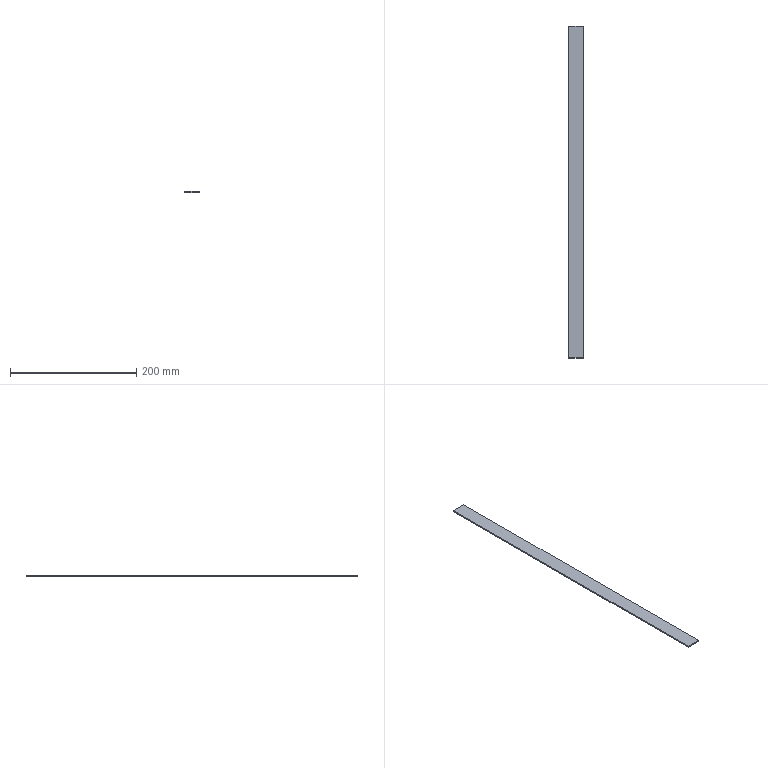Part | SolidWorks | features FlatPattern 1, SMBaseFlange 1, SheetMetal 1 | 1 solid | 6 faces | box 23 x 526 x 2 mm | volume 24196 mm3 | plane 6
STEP:
#1=CARTESIAN_POINT('',(11.5,-263.,0.));
#2=VERTEX_POINT('',#1);
#3=CARTESIAN_POINT('',(11.5,263.,0.));
#4=VERTEX_POINT('',#3);
#5=CARTESIAN_POINT('',(11.5,-263.,0.));
#6=DIRECTION('',(0.,1.,0.));
#7=VECTOR('',#6,1000.);
#8=LINE('',#5,#7);
#9=EDGE_CURVE('',#2,#4,#8,.T.);
#10=ORIENTED_EDGE('',*,*,#9,.F.);
#11=CARTESIAN_POINT('',(11.5,-263.,-2.));
#12=VERTEX_POINT('',#11);
#13=CARTESIAN_POINT('',(11.5,-263.,-2.));
#14=DIRECTION('',(0.,0.,1.));
#15=VECTOR('',#14,1000.);
#16=LINE('',#13,#15);
#17=EDGE_CURVE('',#12,#2,#16,.T.);
#18=ORIENTED_EDGE('',*,*,#17,.F.);
#19=CARTESIAN_POINT('',(11.5,263.,-2.));
#20=VERTEX_POINT('',#19);
#21=CARTESIAN_POINT('',(11.5,-263.,-2.));
#22=DIRECTION('',(0.,1.,0.));
#23=VECTOR('',#22,1000.);
#24=LINE('',#21,#23);
#25=EDGE_CURVE('',#12,#20,#24,.T.);
#26=ORIENTED_EDGE('',*,*,#25,.T.);
#27=CARTESIAN_POINT('',(11.5,263.,-2.));
#28=DIRECTION('',(0.,0.,1.));
#29=VECTOR('',#28,1000.);
#30=LINE('',#27,#29);
#31=EDGE_CURVE('',#20,#4,#30,.T.);
#32=ORIENTED_EDGE('',*,*,#31,.T.);
#33=EDGE_LOOP('',(#10,#18,#26,#32));
#34=FACE_OUTER_BOUND('',#33,.T.);
#35=CARTESIAN_POINT('',(11.5,-263.,-2.));
#36=DIRECTION('',(1.,0.,0.));
#37=DIRECTION('',(0.,0.,-1.));
#38=AXIS2_PLACEMENT_3D('',#35,#36,#37);
#39=PLANE('',#38);
#40=ADVANCED_FACE('',(#34),#39,.T.);
#41=CARTESIAN_POINT('',(-11.5,-263.,0.));
#42=VERTEX_POINT('',#41);
#43=CARTESIAN_POINT('',(-11.5,-263.,0.));
#44=DIRECTION('',(1.,0.,0.));
#45=VECTOR('',#44,1000.);
#46=LINE('',#43,#45);
#47=EDGE_CURVE('',#42,#2,#46,.T.);
#48=ORIENTED_EDGE('',*,*,#47,.F.);
#49=CARTESIAN_POINT('',(-11.5,-263.,-2.));
#50=VERTEX_POINT('',#49);
#51=CARTESIAN_POINT('',(-11.5,-263.,-2.));
#52=DIRECTION('',(0.,0.,1.));
#53=VECTOR('',#52,1000.);
#54=LINE('',#51,#53);
#55=EDGE_CURVE('',#50,#42,#54,.T.);
#56=ORIENTED_EDGE('',*,*,#55,.F.);
#57=CARTESIAN_POINT('',(-11.5,-263.,-2.));
#58=DIRECTION('',(1.,0.,0.));
#59=VECTOR('',#58,1000.);
#60=LINE('',#57,#59);
#61=EDGE_CURVE('',#50,#12,#60,.T.);
#62=ORIENTED_EDGE('',*,*,#61,.T.);
#63=ORIENTED_EDGE('',*,*,#17,.T.);
#64=EDGE_LOOP('',(#48,#56,#62,#63));
#65=FACE_OUTER_BOUND('',#64,.T.);
#66=CARTESIAN_POINT('',(-11.5,-263.,-2.));
#67=DIRECTION('',(0.,-1.,0.));
#68=DIRECTION('',(0.,0.,-1.));
#69=AXIS2_PLACEMENT_3D('',#66,#67,#68);
#70=PLANE('',#69);
#71=ADVANCED_FACE('',(#65),#70,.T.);
#72=CARTESIAN_POINT('',(-11.5,263.,0.));
#73=VERTEX_POINT('',#72);
#74=CARTESIAN_POINT('',(-11.5,-263.,0.));
#75=DIRECTION('',(0.,-1.,0.));
#76=VECTOR('',#75,1000.);
#77=LINE('',#74,#76);
#78=EDGE_CURVE('',#73,#42,#77,.T.);
#79=ORIENTED_EDGE('',*,*,#78,.F.);
#80=CARTESIAN_POINT('',(-11.5,263.,-2.));
#81=VERTEX_POINT('',#80);
#82=CARTESIAN_POINT('',(-11.5,263.,-2.));
#83=DIRECTION('',(0.,0.,1.));
#84=VECTOR('',#83,1000.);
#85=LINE('',#82,#84);
#86=EDGE_CURVE('',#81,#73,#85,.T.);
#87=ORIENTED_EDGE('',*,*,#86,.F.);
#88=CARTESIAN_POINT('',(-11.5,-263.,-2.));
#89=DIRECTION('',(0.,-1.,0.));
#90=VECTOR('',#89,1000.);
#91=LINE('',#88,#90);
#92=EDGE_CURVE('',#81,#50,#91,.T.);
#93=ORIENTED_EDGE('',*,*,#92,.T.);
#94=ORIENTED_EDGE('',*,*,#55,.T.);
#95=EDGE_LOOP('',(#79,#87,#93,#94));
#96=FACE_OUTER_BOUND('',#95,.T.);
#97=CARTESIAN_POINT('',(-11.5,-263.,-2.));
#98=DIRECTION('',(-1.,0.,0.));
#99=DIRECTION('',(0.,0.,1.));
#100=AXIS2_PLACEMENT_3D('',#97,#98,#99);
#101=PLANE('',#100);
#102=ADVANCED_FACE('',(#96),#101,.T.);
#103=CARTESIAN_POINT('',(-11.5,263.,0.));
#104=DIRECTION('',(-1.,0.,0.));
#105=VECTOR('',#104,1000.);
#106=LINE('',#103,#105);
#107=EDGE_CURVE('',#4,#73,#106,.T.);
#108=ORIENTED_EDGE('',*,*,#107,.F.);
#109=ORIENTED_EDGE('',*,*,#31,.F.);
#110=CARTESIAN_POINT('',(-11.5,263.,-2.));
#111=DIRECTION('',(-1.,0.,0.));
#112=VECTOR('',#111,1000.);
#113=LINE('',#110,#112);
#114=EDGE_CURVE('',#20,#81,#113,.T.);
#115=ORIENTED_EDGE('',*,*,#114,.T.);
#116=ORIENTED_EDGE('',*,*,#86,.T.);
#117=EDGE_LOOP('',(#108,#109,#115,#116));
#118=FACE_OUTER_BOUND('',#117,.T.);
#119=CARTESIAN_POINT('',(-11.5,263.,-2.));
#120=DIRECTION('',(0.,1.,0.));
#121=DIRECTION('',(0.,0.,1.));
#122=AXIS2_PLACEMENT_3D('',#119,#120,#121);
#123=PLANE('',#122);
#124=ADVANCED_FACE('',(#118),#123,.T.);
#125=ORIENTED_EDGE('',*,*,#25,.F.);
#126=ORIENTED_EDGE('',*,*,#61,.F.);
#127=ORIENTED_EDGE('',*,*,#92,.F.);
#128=ORIENTED_EDGE('',*,*,#114,.F.);
#129=EDGE_LOOP('',(#125,#126,#127,#128));
#130=FACE_OUTER_BOUND('',#129,.T.);
#131=CARTESIAN_POINT('',(0.,0.,-2.));
#132=DIRECTION('',(0.,0.,-1.));
#133=DIRECTION('',(-1.,0.,0.));
#134=AXIS2_PLACEMENT_3D('',#131,#132,#133);
#135=PLANE('',#134);
#136=ADVANCED_FACE('',(#130),#135,.T.);
#137=ORIENTED_EDGE('',*,*,#9,.T.);
#138=ORIENTED_EDGE('',*,*,#107,.T.);
#139=ORIENTED_EDGE('',*,*,#78,.T.);
#140=ORIENTED_EDGE('',*,*,#47,.T.);
#141=EDGE_LOOP('',(#137,#138,#139,#140));
#142=FACE_OUTER_BOUND('',#141,.T.);
#143=CARTESIAN_POINT('',(0.,0.,0.));
#144=DIRECTION('',(0.,0.,-1.));
#145=DIRECTION('',(-1.,0.,0.));
#146=AXIS2_PLACEMENT_3D('',#143,#144,#145);
#147=PLANE('',#146);
#148=ADVANCED_FACE('',(#142),#147,.F.);
#149=CLOSED_SHELL('',(#40,#71,#102,#124,#136,#148));
#150=MANIFOLD_SOLID_BREP('',#149);
#151=CARTESIAN_POINT('',(0.,0.,0.));
#152=DIRECTION('',(0.,0.,1.));
#153=DIRECTION('',(1.,0.,0.));
#154=AXIS2_PLACEMENT_3D('',#151,#152,#153);
#155=(LENGTH_UNIT()NAMED_UNIT(*)SI_UNIT(.MILLI.,.METRE.));
#156=UNCERTAINTY_MEASURE_WITH_UNIT(LENGTH_MEASURE(0.00001),#155,'','');
#157=(NAMED_UNIT(*)PLANE_ANGLE_UNIT()SI_UNIT($,.RADIAN.));
#158=(NAMED_UNIT(*)SI_UNIT($,.STERADIAN.)SOLID_ANGLE_UNIT());
#159=(GEOMETRIC_REPRESENTATION_CONTEXT(3)GLOBAL_UNCERTAINTY_ASSIGNED_CONTEXT((#156))GLOBAL_UNIT_ASSIGNED_CONTEXT((#155,#157,#158))REPRESENTATION_CONTEXT('',''));
#160=ADVANCED_BREP_SHAPE_REPRESENTATION('',(#150,#154),#159);